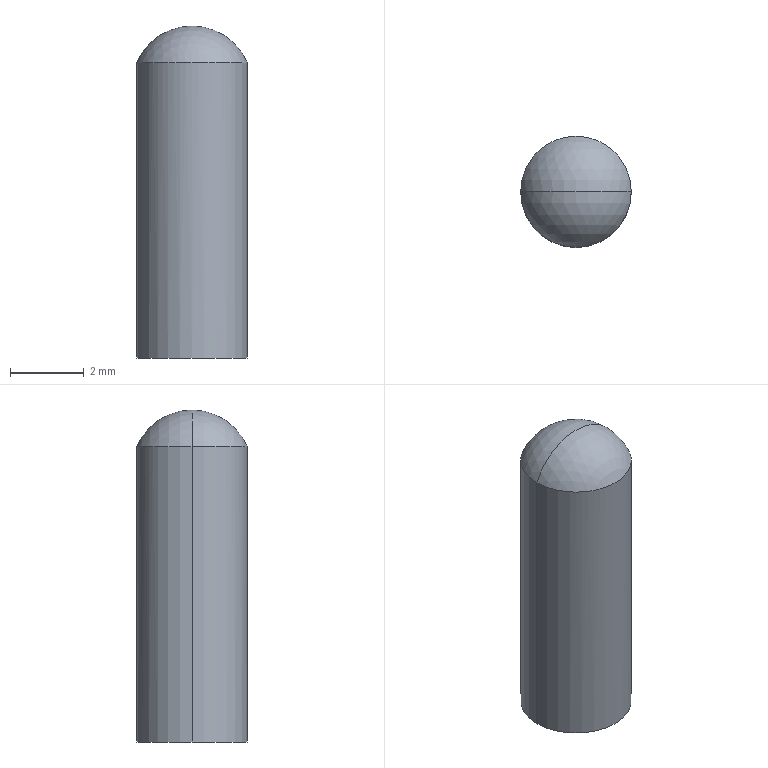Part | STEP file | s3mm pin | 1 solid | 5 faces | box 3 x 3 x 9 mm | volume 60.607 mm3 | sphere 2 | cylinder 2 | plane 1 | commonest cylinder face diameters 3 x2
STEP:
#1=CARTESIAN_POINT('',(0.,0.,0.));
#2=DIRECTION('',(0.,0.,1.));
#3=DIRECTION('',(1.,0.,0.));
#4=AXIS2_PLACEMENT_3D('',#1,#2,#3);
#5=CARTESIAN_POINT('',(1.5,0.,8.));
#6=VERTEX_POINT('',#5);
#7=CARTESIAN_POINT('',(-1.5,0.,8.));
#8=VERTEX_POINT('',#7);
#9=CARTESIAN_POINT('',(0.,0.,8.));
#10=DIRECTION('',(0.,0.,1.));
#11=DIRECTION('',(1.,0.,0.));
#12=AXIS2_PLACEMENT_3D('',#9,#10,#11);
#13=CIRCLE('',#12,1.5);
#14=CARTESIAN_POINT('',(0.,0.,7.375));
#15=DIRECTION('',(0.,1.,0.));
#16=DIRECTION('',(1.,0.,0.));
#17=AXIS2_PLACEMENT_3D('',#14,#15,#16);
#18=SPHERICAL_SURFACE('',#17,1.625);
#19=CARTESIAN_POINT('',(5.888,0.));
#20=CARTESIAN_POINT('',(5.888,0.04393));
#21=CARTESIAN_POINT('',(5.886,0.1318));
#22=CARTESIAN_POINT('',(5.875,0.2632));
#23=CARTESIAN_POINT('',(5.855,0.3938));
#24=CARTESIAN_POINT('',(5.826,0.5229));
#25=CARTESIAN_POINT('',(5.782,0.6497));
#26=CARTESIAN_POINT('',(5.721,0.773));
#27=CARTESIAN_POINT('',(5.633,0.8907));
#28=CARTESIAN_POINT('',(5.506,0.9992));
#29=CARTESIAN_POINT('',(5.32,1.092));
#30=CARTESIAN_POINT('',(5.054,1.159));
#31=CARTESIAN_POINT('',(4.712,1.184));
#32=CARTESIAN_POINT('',(4.371,1.159));
#33=CARTESIAN_POINT('',(4.104,1.092));
#34=CARTESIAN_POINT('',(3.919,0.9992));
#35=CARTESIAN_POINT('',(3.792,0.8907));
#36=CARTESIAN_POINT('',(3.704,0.773));
#37=CARTESIAN_POINT('',(3.642,0.6497));
#38=CARTESIAN_POINT('',(3.599,0.5229));
#39=CARTESIAN_POINT('',(3.569,0.3938));
#40=CARTESIAN_POINT('',(3.55,0.2632));
#41=CARTESIAN_POINT('',(3.539,0.1318));
#42=CARTESIAN_POINT('',(3.536,0.04393));
#43=CARTESIAN_POINT('',(3.536,0.));
#44=B_SPLINE_CURVE_WITH_KNOTS('',3,(#19,#20,#21,#22,#23,#24,#25,#26,#27,#28,#29,#30,#31,#32,#33,#34,#35,#36,#37,#38,#39,#40,#41,#42,#43),.UNSPECIFIED.,.F.,.F.,(4,1,1,1,1,1,1,1,1,1,1,1,1,1,1,1,1,1,1,1,1,1,4),(0.,0.1428,0.2856,0.4284,0.5712,0.714,0.8568,0.9996,1.142,1.285,1.428,1.571,1.714,1.856,1.999,2.142,2.285,2.428,2.57,2.713,2.856,2.999,3.142),.QUASI_UNIFORM_KNOTS.);
#45=(GEOMETRIC_REPRESENTATION_CONTEXT(2)PARAMETRIC_REPRESENTATION_CONTEXT()REPRESENTATION_CONTEXT('',''));
#46=DEFINITIONAL_REPRESENTATION('',(#44),#45);
#47=PCURVE('',#18,#46);
#48=CARTESIAN_POINT('',(0.,0.,8.));
#49=DIRECTION('',(0.,0.,-1.));
#50=DIRECTION('',(-1.,0.,0.));
#51=AXIS2_PLACEMENT_3D('',#48,#49,#50);
#52=CYLINDRICAL_SURFACE('',#51,1.5);
#53=CARTESIAN_POINT('',(3.142,0.));
#54=DIRECTION('',(-1.,0.));
#55=VECTOR('',#54,1.);
#56=LINE('',#53,#55);
#57=(GEOMETRIC_REPRESENTATION_CONTEXT(2)PARAMETRIC_REPRESENTATION_CONTEXT()REPRESENTATION_CONTEXT('',''));
#58=DEFINITIONAL_REPRESENTATION('',(#56),#57);
#59=PCURVE('',#52,#58);
#60=SURFACE_CURVE('',#13,(#47,#59),.PCURVE_S1.);
#61=EDGE_CURVE('',#6,#8,#60,.T.);
#62=ORIENTED_EDGE('',*,*,#61,.T.);
#63=CARTESIAN_POINT('',(0.,0.,9.));
#64=VERTEX_POINT('',#63);
#65=CARTESIAN_POINT('',(0.,0.,7.375));
#66=DIRECTION('',(0.,1.,0.));
#67=DIRECTION('',(-1.,0.,0.));
#68=AXIS2_PLACEMENT_3D('',#65,#66,#67);
#69=CIRCLE('',#68,1.625);
#70=CARTESIAN_POINT('',(3.142,0.));
#71=DIRECTION('',(1.,0.));
#72=VECTOR('',#71,1.);
#73=LINE('',#70,#72);
#74=(GEOMETRIC_REPRESENTATION_CONTEXT(2)PARAMETRIC_REPRESENTATION_CONTEXT()REPRESENTATION_CONTEXT('',''));
#75=DEFINITIONAL_REPRESENTATION('',(#73),#74);
#76=PCURVE('',#18,#75);
#77=CARTESIAN_POINT('',(0.,0.,7.375));
#78=DIRECTION('',(0.,1.,0.));
#79=DIRECTION('',(1.,0.,0.));
#80=AXIS2_PLACEMENT_3D('',#77,#78,#79);
#81=SPHERICAL_SURFACE('',#80,1.625);
#82=CARTESIAN_POINT('',(3.142,0.));
#83=DIRECTION('',(1.,0.));
#84=VECTOR('',#83,1.);
#85=LINE('',#82,#84);
#86=(GEOMETRIC_REPRESENTATION_CONTEXT(2)PARAMETRIC_REPRESENTATION_CONTEXT()REPRESENTATION_CONTEXT('',''));
#87=DEFINITIONAL_REPRESENTATION('',(#85),#86);
#88=PCURVE('',#81,#87);
#89=SURFACE_CURVE('',#69,(#76,#88),.PCURVE_S1.);
#90=EDGE_CURVE('',#8,#64,#89,.T.);
#91=ORIENTED_EDGE('',*,*,#90,.T.);
#92=CARTESIAN_POINT('',(0.,0.,7.375));
#93=DIRECTION('',(0.,-1.,0.));
#94=DIRECTION('',(0.,0.,-1.));
#95=AXIS2_PLACEMENT_3D('',#92,#93,#94);
#96=CIRCLE('',#95,1.625);
#97=CARTESIAN_POINT('',(7.854,0.));
#98=DIRECTION('',(-1.,0.));
#99=VECTOR('',#98,1.);
#100=LINE('',#97,#99);
#101=(GEOMETRIC_REPRESENTATION_CONTEXT(2)PARAMETRIC_REPRESENTATION_CONTEXT()REPRESENTATION_CONTEXT('',''));
#102=DEFINITIONAL_REPRESENTATION('',(#100),#101);
#103=PCURVE('',#18,#102);
#104=CARTESIAN_POINT('',(7.854,0.));
#105=DIRECTION('',(-1.,0.));
#106=VECTOR('',#105,1.);
#107=LINE('',#104,#106);
#108=(GEOMETRIC_REPRESENTATION_CONTEXT(2)PARAMETRIC_REPRESENTATION_CONTEXT()REPRESENTATION_CONTEXT('',''));
#109=DEFINITIONAL_REPRESENTATION('',(#107),#108);
#110=PCURVE('',#81,#109);
#111=SURFACE_CURVE('',#96,(#103,#110),.PCURVE_S1.);
#112=EDGE_CURVE('',#6,#64,#111,.T.);
#113=ORIENTED_EDGE('',*,*,#112,.F.);
#114=EDGE_LOOP('',(#62,#91,#113));
#115=FACE_BOUND('',#114,.T.);
#116=ADVANCED_FACE('',(#115),#18,.T.);
#117=ORIENTED_EDGE('',*,*,#61,.F.);
#118=CARTESIAN_POINT('',(1.5,0.,0.));
#119=VERTEX_POINT('',#118);
#120=CARTESIAN_POINT('',(1.5,0.,8.));
#121=DIRECTION('',(0.,0.,-1.));
#122=VECTOR('',#121,1.);
#123=LINE('',#120,#122);
#124=CARTESIAN_POINT('',(3.142,0.));
#125=DIRECTION('',(0.,1.));
#126=VECTOR('',#125,1.);
#127=LINE('',#124,#126);
#128=(GEOMETRIC_REPRESENTATION_CONTEXT(2)PARAMETRIC_REPRESENTATION_CONTEXT()REPRESENTATION_CONTEXT('',''));
#129=DEFINITIONAL_REPRESENTATION('',(#127),#128);
#130=PCURVE('',#52,#129);
#131=CARTESIAN_POINT('',(0.,0.,8.));
#132=DIRECTION('',(0.,0.,-1.));
#133=DIRECTION('',(-1.,0.,0.));
#134=AXIS2_PLACEMENT_3D('',#131,#132,#133);
#135=CYLINDRICAL_SURFACE('',#134,1.5);
#136=CARTESIAN_POINT('',(3.142,0.));
#137=DIRECTION('',(0.,1.));
#138=VECTOR('',#137,1.);
#139=LINE('',#136,#138);
#140=(GEOMETRIC_REPRESENTATION_CONTEXT(2)PARAMETRIC_REPRESENTATION_CONTEXT()REPRESENTATION_CONTEXT('',''));
#141=DEFINITIONAL_REPRESENTATION('',(#139),#140);
#142=PCURVE('',#135,#141);
#143=SURFACE_CURVE('',#123,(#130,#142),.PCURVE_S1.);
#144=EDGE_CURVE('',#6,#119,#143,.T.);
#145=ORIENTED_EDGE('',*,*,#144,.T.);
#146=CARTESIAN_POINT('',(-1.5,0.,0.));
#147=VERTEX_POINT('',#146);
#148=CARTESIAN_POINT('',(0.,0.,0.));
#149=DIRECTION('',(0.,0.,1.));
#150=DIRECTION('',(1.,0.,0.));
#151=AXIS2_PLACEMENT_3D('',#148,#149,#150);
#152=CIRCLE('',#151,1.5);
#153=CARTESIAN_POINT('',(3.142,8.));
#154=DIRECTION('',(-1.,0.));
#155=VECTOR('',#154,1.);
#156=LINE('',#153,#155);
#157=(GEOMETRIC_REPRESENTATION_CONTEXT(2)PARAMETRIC_REPRESENTATION_CONTEXT()REPRESENTATION_CONTEXT('',''));
#158=DEFINITIONAL_REPRESENTATION('',(#156),#157);
#159=PCURVE('',#52,#158);
#160=CARTESIAN_POINT('',(0.,0.,0.));
#161=DIRECTION('',(0.,0.,1.));
#162=DIRECTION('',(1.,0.,0.));
#163=AXIS2_PLACEMENT_3D('',#160,#161,#162);
#164=PLANE('',#163);
#165=CARTESIAN_POINT('',(0.,0.));
#166=DIRECTION('',(1.,0.));
#167=AXIS2_PLACEMENT_2D('',#165,#166);
#168=CIRCLE('',#167,1.5);
#169=(GEOMETRIC_REPRESENTATION_CONTEXT(2)PARAMETRIC_REPRESENTATION_CONTEXT()REPRESENTATION_CONTEXT('',''));
#170=DEFINITIONAL_REPRESENTATION('',(#168),#169);
#171=PCURVE('',#164,#170);
#172=SURFACE_CURVE('',#152,(#159,#171),.PCURVE_S1.);
#173=EDGE_CURVE('',#119,#147,#172,.T.);
#174=ORIENTED_EDGE('',*,*,#173,.T.);
#175=CARTESIAN_POINT('',(-1.5,0.,8.));
#176=DIRECTION('',(0.,0.,-1.));
#177=VECTOR('',#176,1.);
#178=LINE('',#175,#177);
#179=CARTESIAN_POINT('',(0.,0.));
#180=DIRECTION('',(0.,1.));
#181=VECTOR('',#180,1.);
#182=LINE('',#179,#181);
#183=(GEOMETRIC_REPRESENTATION_CONTEXT(2)PARAMETRIC_REPRESENTATION_CONTEXT()REPRESENTATION_CONTEXT('',''));
#184=DEFINITIONAL_REPRESENTATION('',(#182),#183);
#185=PCURVE('',#52,#184);
#186=CARTESIAN_POINT('',(6.283,0.));
#187=DIRECTION('',(0.,1.));
#188=VECTOR('',#187,1.);
#189=LINE('',#186,#188);
#190=(GEOMETRIC_REPRESENTATION_CONTEXT(2)PARAMETRIC_REPRESENTATION_CONTEXT()REPRESENTATION_CONTEXT('',''));
#191=DEFINITIONAL_REPRESENTATION('',(#189),#190);
#192=PCURVE('',#135,#191);
#193=SURFACE_CURVE('',#178,(#185,#192),.PCURVE_S1.);
#194=EDGE_CURVE('',#8,#147,#193,.T.);
#195=ORIENTED_EDGE('',*,*,#194,.F.);
#196=EDGE_LOOP('',(#117,#145,#174,#195));
#197=FACE_BOUND('',#196,.T.);
#198=ADVANCED_FACE('',(#197),#52,.T.);
#199=ORIENTED_EDGE('',*,*,#144,.F.);
#200=CARTESIAN_POINT('',(0.,0.,8.));
#201=DIRECTION('',(0.,0.,1.));
#202=DIRECTION('',(1.,0.,0.));
#203=AXIS2_PLACEMENT_3D('',#200,#201,#202);
#204=CIRCLE('',#203,1.5);
#205=CARTESIAN_POINT('',(9.425,0.));
#206=DIRECTION('',(-1.,0.));
#207=VECTOR('',#206,1.);
#208=LINE('',#205,#207);
#209=(GEOMETRIC_REPRESENTATION_CONTEXT(2)PARAMETRIC_REPRESENTATION_CONTEXT()REPRESENTATION_CONTEXT('',''));
#210=DEFINITIONAL_REPRESENTATION('',(#208),#209);
#211=PCURVE('',#135,#210);
#212=CARTESIAN_POINT('',(3.536,0.));
#213=CARTESIAN_POINT('',(3.536,-0.04393));
#214=CARTESIAN_POINT('',(3.539,-0.1318));
#215=CARTESIAN_POINT('',(3.55,-0.2632));
#216=CARTESIAN_POINT('',(3.569,-0.3938));
#217=CARTESIAN_POINT('',(3.599,-0.5229));
#218=CARTESIAN_POINT('',(3.642,-0.6497));
#219=CARTESIAN_POINT('',(3.704,-0.773));
#220=CARTESIAN_POINT('',(3.792,-0.8907));
#221=CARTESIAN_POINT('',(3.919,-0.9992));
#222=CARTESIAN_POINT('',(4.104,-1.092));
#223=CARTESIAN_POINT('',(4.371,-1.159));
#224=CARTESIAN_POINT('',(4.712,-1.184));
#225=CARTESIAN_POINT('',(5.054,-1.159));
#226=CARTESIAN_POINT('',(5.32,-1.092));
#227=CARTESIAN_POINT('',(5.506,-0.9992));
#228=CARTESIAN_POINT('',(5.633,-0.8907));
#229=CARTESIAN_POINT('',(5.721,-0.773));
#230=CARTESIAN_POINT('',(5.782,-0.6497));
#231=CARTESIAN_POINT('',(5.826,-0.5229));
#232=CARTESIAN_POINT('',(5.855,-0.3938));
#233=CARTESIAN_POINT('',(5.875,-0.2632));
#234=CARTESIAN_POINT('',(5.886,-0.1318));
#235=CARTESIAN_POINT('',(5.888,-0.04393));
#236=CARTESIAN_POINT('',(5.888,0.));
#237=B_SPLINE_CURVE_WITH_KNOTS('',3,(#212,#213,#214,#215,#216,#217,#218,#219,#220,#221,#222,#223,#224,#225,#226,#227,#228,#229,#230,#231,#232,#233,#234,#235,#236),.UNSPECIFIED.,.F.,.F.,(4,1,1,1,1,1,1,1,1,1,1,1,1,1,1,1,1,1,1,1,1,1,4),(3.142,3.284,3.427,3.57,3.713,3.856,3.998,4.141,4.284,4.427,4.57,4.712,4.855,4.998,5.141,5.284,5.426,5.569,5.712,5.855,5.998,6.14,6.283),.QUASI_UNIFORM_KNOTS.);
#238=(GEOMETRIC_REPRESENTATION_CONTEXT(2)PARAMETRIC_REPRESENTATION_CONTEXT()REPRESENTATION_CONTEXT('',''));
#239=DEFINITIONAL_REPRESENTATION('',(#237),#238);
#240=PCURVE('',#81,#239);
#241=SURFACE_CURVE('',#204,(#211,#240),.PCURVE_S1.);
#242=EDGE_CURVE('',#8,#6,#241,.T.);
#243=ORIENTED_EDGE('',*,*,#242,.F.);
#244=ORIENTED_EDGE('',*,*,#194,.T.);
#245=CARTESIAN_POINT('',(0.,0.,0.));
#246=DIRECTION('',(0.,0.,1.));
#247=DIRECTION('',(1.,0.,0.));
#248=AXIS2_PLACEMENT_3D('',#245,#246,#247);
#249=CIRCLE('',#248,1.5);
#250=CARTESIAN_POINT('',(9.425,8.));
#251=DIRECTION('',(-1.,0.));
#252=VECTOR('',#251,1.);
#253=LINE('',#250,#252);
#254=(GEOMETRIC_REPRESENTATION_CONTEXT(2)PARAMETRIC_REPRESENTATION_CONTEXT()REPRESENTATION_CONTEXT('',''));
#255=DEFINITIONAL_REPRESENTATION('',(#253),#254);
#256=PCURVE('',#135,#255);
#257=CARTESIAN_POINT('',(0.,0.));
#258=DIRECTION('',(1.,0.));
#259=AXIS2_PLACEMENT_2D('',#257,#258);
#260=CIRCLE('',#259,1.5);
#261=(GEOMETRIC_REPRESENTATION_CONTEXT(2)PARAMETRIC_REPRESENTATION_CONTEXT()REPRESENTATION_CONTEXT('',''));
#262=DEFINITIONAL_REPRESENTATION('',(#260),#261);
#263=PCURVE('',#164,#262);
#264=SURFACE_CURVE('',#249,(#256,#263),.PCURVE_S1.);
#265=EDGE_CURVE('',#147,#119,#264,.T.);
#266=ORIENTED_EDGE('',*,*,#265,.T.);
#267=EDGE_LOOP('',(#199,#243,#244,#266));
#268=FACE_BOUND('',#267,.T.);
#269=ADVANCED_FACE('',(#268),#135,.T.);
#270=ORIENTED_EDGE('',*,*,#90,.F.);
#271=ORIENTED_EDGE('',*,*,#242,.T.);
#272=ORIENTED_EDGE('',*,*,#112,.T.);
#273=EDGE_LOOP('',(#270,#271,#272));
#274=FACE_BOUND('',#273,.T.);
#275=ADVANCED_FACE('',(#274),#81,.T.);
#276=ORIENTED_EDGE('',*,*,#265,.F.);
#277=ORIENTED_EDGE('',*,*,#173,.F.);
#278=EDGE_LOOP('',(#276,#277));
#279=FACE_BOUND('',#278,.T.);
#280=ADVANCED_FACE('',(#279),#164,.F.);
#281=CLOSED_SHELL('',(#116,#198,#269,#275,#280));
#282=MANIFOLD_SOLID_BREP('',#281);
#283=(LENGTH_UNIT()NAMED_UNIT(*)SI_UNIT(.MILLI.,.METRE.));
#284=UNCERTAINTY_MEASURE_WITH_UNIT(LENGTH_MEASURE(0.0000001),#283,'','');
#285=(NAMED_UNIT(*)PLANE_ANGLE_UNIT()SI_UNIT($,.RADIAN.));
#286=(NAMED_UNIT(*)SI_UNIT($,.STERADIAN.)SOLID_ANGLE_UNIT());
#287=(GEOMETRIC_REPRESENTATION_CONTEXT(3)GLOBAL_UNCERTAINTY_ASSIGNED_CONTEXT((#284))GLOBAL_UNIT_ASSIGNED_CONTEXT((#283,#285,#286))REPRESENTATION_CONTEXT('',''));
#288=ADVANCED_BREP_SHAPE_REPRESENTATION('',(#4,#282),#287);